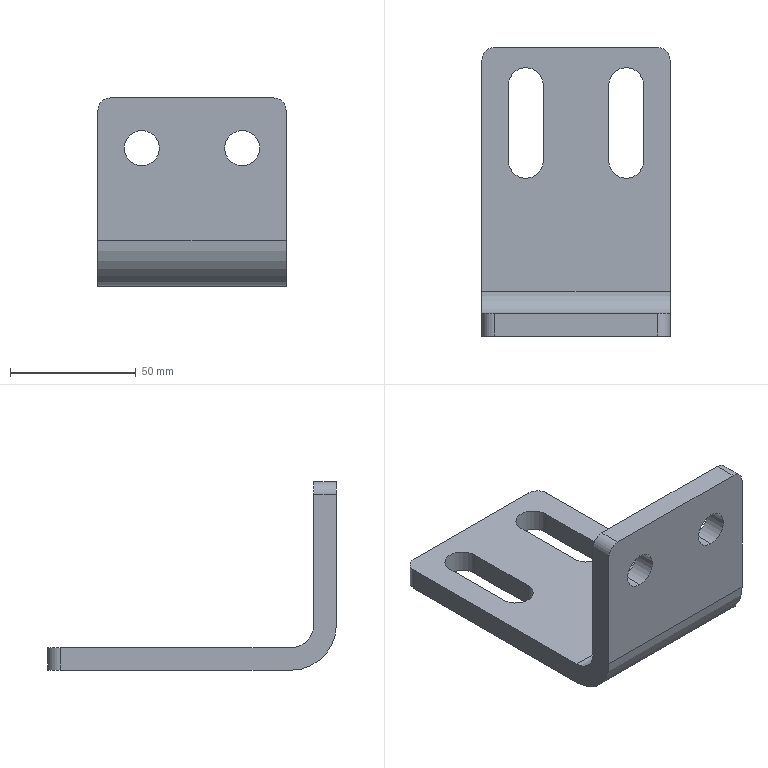Part | STEP file | J451-EBZ05-08-00-Part-1 | 1 solid | 26 faces | box 75 x 115 x 75 mm | volume 104969 mm3 | cylinder 14 | plane 12 | commonest cylinder face diameters 14 x8 10 x4 18 x1 36 x1